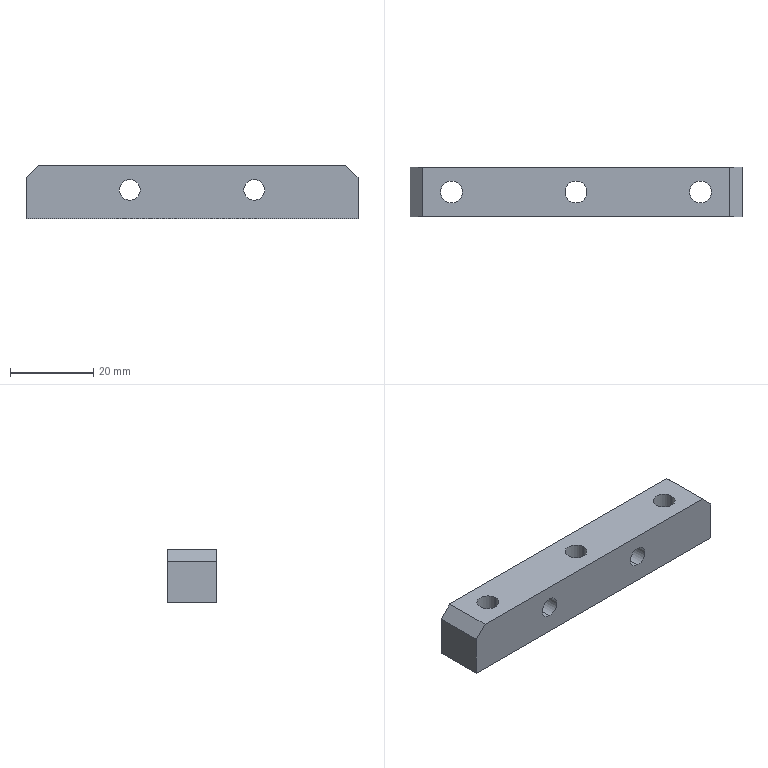Part | STEP file | PN_0013 | 1 solid | 18 faces | box 80 x 12 x 13 mm | volume 11040 mm3 | cylinder 10 | plane 8 | commonest cylinder face diameters 5.3 x6 5 x4
STEP:
#1=CARTESIAN_POINT('',(0.,0.,0.));
#2=DIRECTION('',(0.,0.,1.));
#3=DIRECTION('',(1.,0.,0.));
#4=AXIS2_PLACEMENT_3D('',#1,#2,#3);
#5=CARTESIAN_POINT('',(-15.,0.,3.));
#6=VERTEX_POINT('',#5);
#7=CARTESIAN_POINT('',(-15.,12.,3.));
#8=VERTEX_POINT('',#7);
#9=CARTESIAN_POINT('',(-15.,12.,3.));
#10=DIRECTION('',(0.,1.,0.));
#11=VECTOR('',#10,1.);
#12=LINE('',#9,#11);
#13=CARTESIAN_POINT('',(-15.,12.,0.5));
#14=DIRECTION('',(0.,1.,0.));
#15=DIRECTION('',(0.,0.,1.));
#16=AXIS2_PLACEMENT_3D('',#13,#14,#15);
#17=CYLINDRICAL_SURFACE('',#16,2.5);
#18=CARTESIAN_POINT('',(6.283,0.));
#19=DIRECTION('',(0.,1.));
#20=VECTOR('',#19,1.);
#21=LINE('',#18,#20);
#22=(GEOMETRIC_REPRESENTATION_CONTEXT(2)PARAMETRIC_REPRESENTATION_CONTEXT()REPRESENTATION_CONTEXT('',''));
#23=DEFINITIONAL_REPRESENTATION('',(#21),#22);
#24=PCURVE('',#17,#23);
#25=CARTESIAN_POINT('',(-15.,12.,0.5));
#26=DIRECTION('',(0.,1.,0.));
#27=DIRECTION('',(0.,0.,1.));
#28=AXIS2_PLACEMENT_3D('',#25,#26,#27);
#29=CYLINDRICAL_SURFACE('',#28,2.5);
#30=CARTESIAN_POINT('',(0.,0.));
#31=DIRECTION('',(0.,1.));
#32=VECTOR('',#31,1.);
#33=LINE('',#30,#32);
#34=(GEOMETRIC_REPRESENTATION_CONTEXT(2)PARAMETRIC_REPRESENTATION_CONTEXT()REPRESENTATION_CONTEXT('',''));
#35=DEFINITIONAL_REPRESENTATION('',(#33),#34);
#36=PCURVE('',#29,#35);
#37=SURFACE_CURVE('',#12,(#24,#36),.PCURVE_S1.);
#38=EDGE_CURVE('',#6,#8,#37,.T.);
#39=ORIENTED_EDGE('',*,*,#38,.T.);
#40=CARTESIAN_POINT('',(-15.,12.,-2.));
#41=VERTEX_POINT('',#40);
#42=CARTESIAN_POINT('',(-15.,12.,0.5));
#43=DIRECTION('',(0.,1.,0.));
#44=DIRECTION('',(0.,0.,1.));
#45=AXIS2_PLACEMENT_3D('',#42,#43,#44);
#46=CIRCLE('',#45,2.5);
#47=CARTESIAN_POINT('',(0.,0.));
#48=DIRECTION('',(1.,0.));
#49=VECTOR('',#48,1.);
#50=LINE('',#47,#49);
#51=(GEOMETRIC_REPRESENTATION_CONTEXT(2)PARAMETRIC_REPRESENTATION_CONTEXT()REPRESENTATION_CONTEXT('',''));
#52=DEFINITIONAL_REPRESENTATION('',(#50),#51);
#53=PCURVE('',#17,#52);
#54=CARTESIAN_POINT('',(0.,12.,0.));
#55=DIRECTION('',(0.,1.,0.));
#56=DIRECTION('',(0.,0.,1.));
#57=AXIS2_PLACEMENT_3D('',#54,#55,#56);
#58=PLANE('',#57);
#59=CARTESIAN_POINT('',(0.5,-15.));
#60=DIRECTION('',(1.,0.));
#61=AXIS2_PLACEMENT_2D('',#59,#60);
#62=CIRCLE('',#61,2.5);
#63=(GEOMETRIC_REPRESENTATION_CONTEXT(2)PARAMETRIC_REPRESENTATION_CONTEXT()REPRESENTATION_CONTEXT('',''));
#64=DEFINITIONAL_REPRESENTATION('',(#62),#63);
#65=PCURVE('',#58,#64);
#66=SURFACE_CURVE('',#46,(#53,#65),.PCURVE_S1.);
#67=EDGE_CURVE('',#41,#8,#66,.T.);
#68=ORIENTED_EDGE('',*,*,#67,.F.);
#69=CARTESIAN_POINT('',(-15.,0.,-2.));
#70=VERTEX_POINT('',#69);
#71=CARTESIAN_POINT('',(-15.,12.,-2.));
#72=DIRECTION('',(0.,1.,0.));
#73=VECTOR('',#72,1.);
#74=LINE('',#71,#73);
#75=CARTESIAN_POINT('',(3.142,0.));
#76=DIRECTION('',(0.,1.));
#77=VECTOR('',#76,1.);
#78=LINE('',#75,#77);
#79=(GEOMETRIC_REPRESENTATION_CONTEXT(2)PARAMETRIC_REPRESENTATION_CONTEXT()REPRESENTATION_CONTEXT('',''));
#80=DEFINITIONAL_REPRESENTATION('',(#78),#79);
#81=PCURVE('',#17,#80);
#82=CARTESIAN_POINT('',(3.142,0.));
#83=DIRECTION('',(0.,1.));
#84=VECTOR('',#83,1.);
#85=LINE('',#82,#84);
#86=(GEOMETRIC_REPRESENTATION_CONTEXT(2)PARAMETRIC_REPRESENTATION_CONTEXT()REPRESENTATION_CONTEXT('',''));
#87=DEFINITIONAL_REPRESENTATION('',(#85),#86);
#88=PCURVE('',#29,#87);
#89=SURFACE_CURVE('',#74,(#81,#88),.PCURVE_S1.);
#90=EDGE_CURVE('',#70,#41,#89,.T.);
#91=ORIENTED_EDGE('',*,*,#90,.F.);
#92=CARTESIAN_POINT('',(-15.,0.,0.5));
#93=DIRECTION('',(0.,1.,0.));
#94=DIRECTION('',(0.,0.,1.));
#95=AXIS2_PLACEMENT_3D('',#92,#93,#94);
#96=CIRCLE('',#95,2.5);
#97=CARTESIAN_POINT('',(0.,-12.));
#98=DIRECTION('',(1.,0.));
#99=VECTOR('',#98,1.);
#100=LINE('',#97,#99);
#101=(GEOMETRIC_REPRESENTATION_CONTEXT(2)PARAMETRIC_REPRESENTATION_CONTEXT()REPRESENTATION_CONTEXT('',''));
#102=DEFINITIONAL_REPRESENTATION('',(#100),#101);
#103=PCURVE('',#17,#102);
#104=CARTESIAN_POINT('',(0.,0.,0.));
#105=DIRECTION('',(0.,1.,0.));
#106=DIRECTION('',(0.,0.,1.));
#107=AXIS2_PLACEMENT_3D('',#104,#105,#106);
#108=PLANE('',#107);
#109=CARTESIAN_POINT('',(0.5,-15.));
#110=DIRECTION('',(1.,0.));
#111=AXIS2_PLACEMENT_2D('',#109,#110);
#112=CIRCLE('',#111,2.5);
#113=(GEOMETRIC_REPRESENTATION_CONTEXT(2)PARAMETRIC_REPRESENTATION_CONTEXT()REPRESENTATION_CONTEXT('',''));
#114=DEFINITIONAL_REPRESENTATION('',(#112),#113);
#115=PCURVE('',#108,#114);
#116=SURFACE_CURVE('',#96,(#103,#115),.PCURVE_S1.);
#117=EDGE_CURVE('',#70,#6,#116,.T.);
#118=ORIENTED_EDGE('',*,*,#117,.T.);
#119=EDGE_LOOP('',(#39,#68,#91,#118));
#120=FACE_BOUND('',#119,.F.);
#121=ADVANCED_FACE('',(#120),#17,.F.);
#122=CARTESIAN_POINT('',(15.,0.,3.));
#123=VERTEX_POINT('',#122);
#124=CARTESIAN_POINT('',(15.,12.,3.));
#125=VERTEX_POINT('',#124);
#126=CARTESIAN_POINT('',(15.,12.,3.));
#127=DIRECTION('',(0.,1.,0.));
#128=VECTOR('',#127,1.);
#129=LINE('',#126,#128);
#130=CARTESIAN_POINT('',(15.,12.,0.5));
#131=DIRECTION('',(0.,1.,0.));
#132=DIRECTION('',(0.,0.,1.));
#133=AXIS2_PLACEMENT_3D('',#130,#131,#132);
#134=CYLINDRICAL_SURFACE('',#133,2.5);
#135=CARTESIAN_POINT('',(6.283,0.));
#136=DIRECTION('',(0.,1.));
#137=VECTOR('',#136,1.);
#138=LINE('',#135,#137);
#139=(GEOMETRIC_REPRESENTATION_CONTEXT(2)PARAMETRIC_REPRESENTATION_CONTEXT()REPRESENTATION_CONTEXT('',''));
#140=DEFINITIONAL_REPRESENTATION('',(#138),#139);
#141=PCURVE('',#134,#140);
#142=CARTESIAN_POINT('',(15.,12.,0.5));
#143=DIRECTION('',(0.,1.,0.));
#144=DIRECTION('',(0.,0.,1.));
#145=AXIS2_PLACEMENT_3D('',#142,#143,#144);
#146=CYLINDRICAL_SURFACE('',#145,2.5);
#147=CARTESIAN_POINT('',(0.,0.));
#148=DIRECTION('',(0.,1.));
#149=VECTOR('',#148,1.);
#150=LINE('',#147,#149);
#151=(GEOMETRIC_REPRESENTATION_CONTEXT(2)PARAMETRIC_REPRESENTATION_CONTEXT()REPRESENTATION_CONTEXT('',''));
#152=DEFINITIONAL_REPRESENTATION('',(#150),#151);
#153=PCURVE('',#146,#152);
#154=SURFACE_CURVE('',#129,(#141,#153),.PCURVE_S1.);
#155=EDGE_CURVE('',#123,#125,#154,.T.);
#156=ORIENTED_EDGE('',*,*,#155,.T.);
#157=CARTESIAN_POINT('',(15.,12.,-2.));
#158=VERTEX_POINT('',#157);
#159=CARTESIAN_POINT('',(15.,12.,0.5));
#160=DIRECTION('',(0.,1.,0.));
#161=DIRECTION('',(0.,0.,1.));
#162=AXIS2_PLACEMENT_3D('',#159,#160,#161);
#163=CIRCLE('',#162,2.5);
#164=CARTESIAN_POINT('',(0.,0.));
#165=DIRECTION('',(1.,0.));
#166=VECTOR('',#165,1.);
#167=LINE('',#164,#166);
#168=(GEOMETRIC_REPRESENTATION_CONTEXT(2)PARAMETRIC_REPRESENTATION_CONTEXT()REPRESENTATION_CONTEXT('',''));
#169=DEFINITIONAL_REPRESENTATION('',(#167),#168);
#170=PCURVE('',#134,#169);
#171=CARTESIAN_POINT('',(0.5,15.));
#172=DIRECTION('',(1.,0.));
#173=AXIS2_PLACEMENT_2D('',#171,#172);
#174=CIRCLE('',#173,2.5);
#175=(GEOMETRIC_REPRESENTATION_CONTEXT(2)PARAMETRIC_REPRESENTATION_CONTEXT()REPRESENTATION_CONTEXT('',''));
#176=DEFINITIONAL_REPRESENTATION('',(#174),#175);
#177=PCURVE('',#58,#176);
#178=SURFACE_CURVE('',#163,(#170,#177),.PCURVE_S1.);
#179=EDGE_CURVE('',#158,#125,#178,.T.);
#180=ORIENTED_EDGE('',*,*,#179,.F.);
#181=CARTESIAN_POINT('',(15.,0.,-2.));
#182=VERTEX_POINT('',#181);
#183=CARTESIAN_POINT('',(15.,12.,-2.));
#184=DIRECTION('',(0.,1.,0.));
#185=VECTOR('',#184,1.);
#186=LINE('',#183,#185);
#187=CARTESIAN_POINT('',(3.142,0.));
#188=DIRECTION('',(0.,1.));
#189=VECTOR('',#188,1.);
#190=LINE('',#187,#189);
#191=(GEOMETRIC_REPRESENTATION_CONTEXT(2)PARAMETRIC_REPRESENTATION_CONTEXT()REPRESENTATION_CONTEXT('',''));
#192=DEFINITIONAL_REPRESENTATION('',(#190),#191);
#193=PCURVE('',#134,#192);
#194=CARTESIAN_POINT('',(3.142,0.));
#195=DIRECTION('',(0.,1.));
#196=VECTOR('',#195,1.);
#197=LINE('',#194,#196);
#198=(GEOMETRIC_REPRESENTATION_CONTEXT(2)PARAMETRIC_REPRESENTATION_CONTEXT()REPRESENTATION_CONTEXT('',''));
#199=DEFINITIONAL_REPRESENTATION('',(#197),#198);
#200=PCURVE('',#146,#199);
#201=SURFACE_CURVE('',#186,(#193,#200),.PCURVE_S1.);
#202=EDGE_CURVE('',#182,#158,#201,.T.);
#203=ORIENTED_EDGE('',*,*,#202,.F.);
#204=CARTESIAN_POINT('',(15.,0.,0.5));
#205=DIRECTION('',(0.,1.,0.));
#206=DIRECTION('',(0.,0.,1.));
#207=AXIS2_PLACEMENT_3D('',#204,#205,#206);
#208=CIRCLE('',#207,2.5);
#209=CARTESIAN_POINT('',(0.,-12.));
#210=DIRECTION('',(1.,0.));
#211=VECTOR('',#210,1.);
#212=LINE('',#209,#211);
#213=(GEOMETRIC_REPRESENTATION_CONTEXT(2)PARAMETRIC_REPRESENTATION_CONTEXT()REPRESENTATION_CONTEXT('',''));
#214=DEFINITIONAL_REPRESENTATION('',(#212),#213);
#215=PCURVE('',#134,#214);
#216=CARTESIAN_POINT('',(0.5,15.));
#217=DIRECTION('',(1.,0.));
#218=AXIS2_PLACEMENT_2D('',#216,#217);
#219=CIRCLE('',#218,2.5);
#220=(GEOMETRIC_REPRESENTATION_CONTEXT(2)PARAMETRIC_REPRESENTATION_CONTEXT()REPRESENTATION_CONTEXT('',''));
#221=DEFINITIONAL_REPRESENTATION('',(#219),#220);
#222=PCURVE('',#108,#221);
#223=SURFACE_CURVE('',#208,(#215,#222),.PCURVE_S1.);
#224=EDGE_CURVE('',#182,#123,#223,.T.);
#225=ORIENTED_EDGE('',*,*,#224,.T.);
#226=EDGE_LOOP('',(#156,#180,#203,#225));
#227=FACE_BOUND('',#226,.F.);
#228=ADVANCED_FACE('',(#227),#134,.F.);
#229=CARTESIAN_POINT('',(32.65,6.,-6.5));
#230=VERTEX_POINT('',#229);
#231=CARTESIAN_POINT('',(32.65,6.,6.5));
#232=VERTEX_POINT('',#231);
#233=CARTESIAN_POINT('',(32.65,6.,6.5));
#234=DIRECTION('',(0.,0.,1.));
#235=VECTOR('',#234,1.);
#236=LINE('',#233,#235);
#237=CARTESIAN_POINT('',(30.,6.,6.5));
#238=DIRECTION('',(0.,0.,1.));
#239=DIRECTION('',(1.,0.,0.));
#240=AXIS2_PLACEMENT_3D('',#237,#238,#239);
#241=CYLINDRICAL_SURFACE('',#240,2.65);
#242=CARTESIAN_POINT('',(6.283,0.));
#243=DIRECTION('',(0.,1.));
#244=VECTOR('',#243,1.);
#245=LINE('',#242,#244);
#246=(GEOMETRIC_REPRESENTATION_CONTEXT(2)PARAMETRIC_REPRESENTATION_CONTEXT()REPRESENTATION_CONTEXT('',''));
#247=DEFINITIONAL_REPRESENTATION('',(#245),#246);
#248=PCURVE('',#241,#247);
#249=CARTESIAN_POINT('',(30.,6.,6.5));
#250=DIRECTION('',(0.,0.,1.));
#251=DIRECTION('',(1.,0.,0.));
#252=AXIS2_PLACEMENT_3D('',#249,#250,#251);
#253=CYLINDRICAL_SURFACE('',#252,2.65);
#254=CARTESIAN_POINT('',(0.,0.));
#255=DIRECTION('',(0.,1.));
#256=VECTOR('',#255,1.);
#257=LINE('',#254,#256);
#258=(GEOMETRIC_REPRESENTATION_CONTEXT(2)PARAMETRIC_REPRESENTATION_CONTEXT()REPRESENTATION_CONTEXT('',''));
#259=DEFINITIONAL_REPRESENTATION('',(#257),#258);
#260=PCURVE('',#253,#259);
#261=SURFACE_CURVE('',#236,(#248,#260),.PCURVE_S1.);
#262=EDGE_CURVE('',#230,#232,#261,.T.);
#263=ORIENTED_EDGE('',*,*,#262,.T.);
#264=CARTESIAN_POINT('',(27.35,6.,6.5));
#265=VERTEX_POINT('',#264);
#266=CARTESIAN_POINT('',(30.,6.,6.5));
#267=DIRECTION('',(0.,0.,1.));
#268=DIRECTION('',(1.,0.,0.));
#269=AXIS2_PLACEMENT_3D('',#266,#267,#268);
#270=CIRCLE('',#269,2.65);
#271=CARTESIAN_POINT('',(0.,0.));
#272=DIRECTION('',(1.,0.));
#273=VECTOR('',#272,1.);
#274=LINE('',#271,#273);
#275=(GEOMETRIC_REPRESENTATION_CONTEXT(2)PARAMETRIC_REPRESENTATION_CONTEXT()REPRESENTATION_CONTEXT('',''));
#276=DEFINITIONAL_REPRESENTATION('',(#274),#275);
#277=PCURVE('',#241,#276);
#278=CARTESIAN_POINT('',(-40.,12.,6.5));
#279=DIRECTION('',(0.,0.,-1.));
#280=DIRECTION('',(-1.,0.,0.));
#281=AXIS2_PLACEMENT_3D('',#278,#279,#280);
#282=PLANE('',#281);
#283=CARTESIAN_POINT('',(-72.65,-6.));
#284=CARTESIAN_POINT('',(-72.65,-1.41));
#285=CARTESIAN_POINT('',(-68.675,-3.705));
#286=CARTESIAN_POINT('',(-64.7,-6.));
#287=CARTESIAN_POINT('',(-68.675,-8.295));
#288=CARTESIAN_POINT('',(-72.65,-10.59));
#289=CARTESIAN_POINT('',(-72.65,-6.));
#290=(BOUNDED_CURVE()B_SPLINE_CURVE(2,(#283,#284,#285,#286,#287,#288,#289),.UNSPECIFIED.,.T.,.F.)B_SPLINE_CURVE_WITH_KNOTS((1,2,2,2,2,1),(-2.094,0.,2.094,4.189,6.283,8.378),.UNSPECIFIED.)CURVE()GEOMETRIC_REPRESENTATION_ITEM()RATIONAL_B_SPLINE_CURVE((1.,0.5,1.,0.5,1.,0.5,1.))REPRESENTATION_ITEM(''));
#291=(GEOMETRIC_REPRESENTATION_CONTEXT(2)PARAMETRIC_REPRESENTATION_CONTEXT()REPRESENTATION_CONTEXT('',''));
#292=DEFINITIONAL_REPRESENTATION('',(#290),#291);
#293=PCURVE('',#282,#292);
#294=SURFACE_CURVE('',#270,(#277,#293),.PCURVE_S1.);
#295=EDGE_CURVE('',#265,#232,#294,.T.);
#296=ORIENTED_EDGE('',*,*,#295,.F.);
#297=CARTESIAN_POINT('',(27.35,6.,-6.5));
#298=VERTEX_POINT('',#297);
#299=CARTESIAN_POINT('',(27.35,6.,6.5));
#300=DIRECTION('',(0.,0.,1.));
#301=VECTOR('',#300,1.);
#302=LINE('',#299,#301);
#303=CARTESIAN_POINT('',(3.142,0.));
#304=DIRECTION('',(0.,1.));
#305=VECTOR('',#304,1.);
#306=LINE('',#303,#305);
#307=(GEOMETRIC_REPRESENTATION_CONTEXT(2)PARAMETRIC_REPRESENTATION_CONTEXT()REPRESENTATION_CONTEXT('',''));
#308=DEFINITIONAL_REPRESENTATION('',(#306),#307);
#309=PCURVE('',#241,#308);
#310=CARTESIAN_POINT('',(3.142,0.));
#311=DIRECTION('',(0.,1.));
#312=VECTOR('',#311,1.);
#313=LINE('',#310,#312);
#314=(GEOMETRIC_REPRESENTATION_CONTEXT(2)PARAMETRIC_REPRESENTATION_CONTEXT()REPRESENTATION_CONTEXT('',''));
#315=DEFINITIONAL_REPRESENTATION('',(#313),#314);
#316=PCURVE('',#253,#315);
#317=SURFACE_CURVE('',#302,(#309,#316),.PCURVE_S1.);
#318=EDGE_CURVE('',#298,#265,#317,.T.);
#319=ORIENTED_EDGE('',*,*,#318,.F.);
#320=CARTESIAN_POINT('',(30.,6.,-6.5));
#321=DIRECTION('',(0.,0.,1.));
#322=DIRECTION('',(1.,0.,0.));
#323=AXIS2_PLACEMENT_3D('',#320,#321,#322);
#324=CIRCLE('',#323,2.65);
#325=CARTESIAN_POINT('',(0.,-13.));
#326=DIRECTION('',(1.,0.));
#327=VECTOR('',#326,1.);
#328=LINE('',#325,#327);
#329=(GEOMETRIC_REPRESENTATION_CONTEXT(2)PARAMETRIC_REPRESENTATION_CONTEXT()REPRESENTATION_CONTEXT('',''));
#330=DEFINITIONAL_REPRESENTATION('',(#328),#329);
#331=PCURVE('',#241,#330);
#332=CARTESIAN_POINT('',(-40.,12.,-6.5));
#333=DIRECTION('',(0.,0.,1.));
#334=DIRECTION('',(1.,0.,0.));
#335=AXIS2_PLACEMENT_3D('',#332,#333,#334);
#336=PLANE('',#335);
#337=CARTESIAN_POINT('',(70.,-6.));
#338=DIRECTION('',(1.,0.));
#339=AXIS2_PLACEMENT_2D('',#337,#338);
#340=CIRCLE('',#339,2.65);
#341=(GEOMETRIC_REPRESENTATION_CONTEXT(2)PARAMETRIC_REPRESENTATION_CONTEXT()REPRESENTATION_CONTEXT('',''));
#342=DEFINITIONAL_REPRESENTATION('',(#340),#341);
#343=PCURVE('',#336,#342);
#344=SURFACE_CURVE('',#324,(#331,#343),.PCURVE_S1.);
#345=EDGE_CURVE('',#298,#230,#344,.T.);
#346=ORIENTED_EDGE('',*,*,#345,.T.);
#347=EDGE_LOOP('',(#263,#296,#319,#346));
#348=FACE_BOUND('',#347,.F.);
#349=ADVANCED_FACE('',(#348),#241,.F.);
#350=CARTESIAN_POINT('',(2.65,6.,-6.5));
#351=VERTEX_POINT('',#350);
#352=CARTESIAN_POINT('',(2.65,6.,6.5));
#353=VERTEX_POINT('',#352);
#354=CARTESIAN_POINT('',(2.65,6.,6.5));
#355=DIRECTION('',(0.,0.,1.));
#356=VECTOR('',#355,1.);
#357=LINE('',#354,#356);
#358=CARTESIAN_POINT('',(0.,6.,6.5));
#359=DIRECTION('',(0.,0.,1.));
#360=DIRECTION('',(1.,0.,0.));
#361=AXIS2_PLACEMENT_3D('',#358,#359,#360);
#362=CYLINDRICAL_SURFACE('',#361,2.65);
#363=CARTESIAN_POINT('',(6.283,0.));
#364=DIRECTION('',(0.,1.));
#365=VECTOR('',#364,1.);
#366=LINE('',#363,#365);
#367=(GEOMETRIC_REPRESENTATION_CONTEXT(2)PARAMETRIC_REPRESENTATION_CONTEXT()REPRESENTATION_CONTEXT('',''));
#368=DEFINITIONAL_REPRESENTATION('',(#366),#367);
#369=PCURVE('',#362,#368);
#370=CARTESIAN_POINT('',(0.,6.,6.5));
#371=DIRECTION('',(0.,0.,1.));
#372=DIRECTION('',(1.,0.,0.));
#373=AXIS2_PLACEMENT_3D('',#370,#371,#372);
#374=CYLINDRICAL_SURFACE('',#373,2.65);
#375=CARTESIAN_POINT('',(0.,0.));
#376=DIRECTION('',(0.,1.));
#377=VECTOR('',#376,1.);
#378=LINE('',#375,#377);
#379=(GEOMETRIC_REPRESENTATION_CONTEXT(2)PARAMETRIC_REPRESENTATION_CONTEXT()REPRESENTATION_CONTEXT('',''));
#380=DEFINITIONAL_REPRESENTATION('',(#378),#379);
#381=PCURVE('',#374,#380);
#382=SURFACE_CURVE('',#357,(#369,#381),.PCURVE_S1.);
#383=EDGE_CURVE('',#351,#353,#382,.T.);
#384=ORIENTED_EDGE('',*,*,#383,.T.);
#385=CARTESIAN_POINT('',(-2.65,6.,6.5));
#386=VERTEX_POINT('',#385);
#387=CARTESIAN_POINT('',(0.,6.,6.5));
#388=DIRECTION('',(0.,0.,1.));
#389=DIRECTION('',(1.,0.,0.));
#390=AXIS2_PLACEMENT_3D('',#387,#388,#389);
#391=CIRCLE('',#390,2.65);
#392=CARTESIAN_POINT('',(0.,0.));
#393=DIRECTION('',(1.,0.));
#394=VECTOR('',#393,1.);
#395=LINE('',#392,#394);
#396=(GEOMETRIC_REPRESENTATION_CONTEXT(2)PARAMETRIC_REPRESENTATION_CONTEXT()REPRESENTATION_CONTEXT('',''));
#397=DEFINITIONAL_REPRESENTATION('',(#395),#396);
#398=PCURVE('',#362,#397);
#399=CARTESIAN_POINT('',(-42.65,-6.));
#400=CARTESIAN_POINT('',(-42.65,-1.41));
#401=CARTESIAN_POINT('',(-38.675,-3.705));
#402=CARTESIAN_POINT('',(-34.7,-6.));
#403=CARTESIAN_POINT('',(-38.675,-8.295));
#404=CARTESIAN_POINT('',(-42.65,-10.59));
#405=CARTESIAN_POINT('',(-42.65,-6.));
#406=(BOUNDED_CURVE()B_SPLINE_CURVE(2,(#399,#400,#401,#402,#403,#404,#405),.UNSPECIFIED.,.T.,.F.)B_SPLINE_CURVE_WITH_KNOTS((1,2,2,2,2,1),(-2.094,0.,2.094,4.189,6.283,8.378),.UNSPECIFIED.)CURVE()GEOMETRIC_REPRESENTATION_ITEM()RATIONAL_B_SPLINE_CURVE((1.,0.5,1.,0.5,1.,0.5,1.))REPRESENTATION_ITEM(''));
#407=(GEOMETRIC_REPRESENTATION_CONTEXT(2)PARAMETRIC_REPRESENTATION_CONTEXT()REPRESENTATION_CONTEXT('',''));
#408=DEFINITIONAL_REPRESENTATION('',(#406),#407);
#409=PCURVE('',#282,#408);
#410=SURFACE_CURVE('',#391,(#398,#409),.PCURVE_S1.);
#411=EDGE_CURVE('',#386,#353,#410,.T.);
#412=ORIENTED_EDGE('',*,*,#411,.F.);
#413=CARTESIAN_POINT('',(-2.65,6.,-6.5));
#414=VERTEX_POINT('',#413);
#415=CARTESIAN_POINT('',(-2.65,6.,6.5));
#416=DIRECTION('',(0.,0.,1.));
#417=VECTOR('',#416,1.);
#418=LINE('',#415,#417);
#419=CARTESIAN_POINT('',(3.142,0.));
#420=DIRECTION('',(0.,1.));
#421=VECTOR('',#420,1.);
#422=LINE('',#419,#421);
#423=(GEOMETRIC_REPRESENTATION_CONTEXT(2)PARAMETRIC_REPRESENTATION_CONTEXT()REPRESENTATION_CONTEXT('',''));
#424=DEFINITIONAL_REPRESENTATION('',(#422),#423);
#425=PCURVE('',#362,#424);
#426=CARTESIAN_POINT('',(3.142,0.));
#427=DIRECTION('',(0.,1.));
#428=VECTOR('',#427,1.);
#429=LINE('',#426,#428);
#430=(GEOMETRIC_REPRESENTATION_CONTEXT(2)PARAMETRIC_REPRESENTATION_CONTEXT()REPRESENTATION_CONTEXT('',''));
#431=DEFINITIONAL_REPRESENTATION('',(#429),#430);
#432=PCURVE('',#374,#431);
#433=SURFACE_CURVE('',#418,(#425,#432),.PCURVE_S1.);
#434=EDGE_CURVE('',#414,#386,#433,.T.);
#435=ORIENTED_EDGE('',*,*,#434,.F.);
#436=CARTESIAN_POINT('',(0.,6.,-6.5));
#437=DIRECTION('',(0.,0.,1.));
#438=DIRECTION('',(1.,0.,0.));
#439=AXIS2_PLACEMENT_3D('',#436,#437,#438);
#440=CIRCLE('',#439,2.65);
#441=CARTESIAN_POINT('',(0.,-13.));
#442=DIRECTION('',(1.,0.));
#443=VECTOR('',#442,1.);
#444=LINE('',#441,#443);
#445=(GEOMETRIC_REPRESENTATION_CONTEXT(2)PARAMETRIC_REPRESENTATION_CONTEXT()REPRESENTATION_CONTEXT('',''));
#446=DEFINITIONAL_REPRESENTATION('',(#444),#445);
#447=PCURVE('',#362,#446);
#448=CARTESIAN_POINT('',(40.,-6.));
#449=DIRECTION('',(1.,0.));
#450=AXIS2_PLACEMENT_2D('',#448,#449);
#451=CIRCLE('',#450,2.65);
#452=(GEOMETRIC_REPRESENTATION_CONTEXT(2)PARAMETRIC_REPRESENTATION_CONTEXT()REPRESENTATION_CONTEXT('',''));
#453=DEFINITIONAL_REPRESENTATION('',(#451),#452);
#454=PCURVE('',#336,#453);
#455=SURFACE_CURVE('',#440,(#447,#454),.PCURVE_S1.);
#456=EDGE_CURVE('',#414,#351,#455,.T.);
#457=ORIENTED_EDGE('',*,*,#456,.T.);
#458=EDGE_LOOP('',(#384,#412,#435,#457));
#459=FACE_BOUND('',#458,.F.);
#460=ADVANCED_FACE('',(#459),#362,.F.);
#461=CARTESIAN_POINT('',(-27.35,6.,-6.5));
#462=VERTEX_POINT('',#461);
#463=CARTESIAN_POINT('',(-27.35,6.,6.5));
#464=VERTEX_POINT('',#463);
#465=CARTESIAN_POINT('',(-27.35,6.,6.5));
#466=DIRECTION('',(0.,0.,1.));
#467=VECTOR('',#466,1.);
#468=LINE('',#465,#467);
#469=CARTESIAN_POINT('',(-30.,6.,6.5));
#470=DIRECTION('',(0.,0.,1.));
#471=DIRECTION('',(1.,0.,0.));
#472=AXIS2_PLACEMENT_3D('',#469,#470,#471);
#473=CYLINDRICAL_SURFACE('',#472,2.65);
#474=CARTESIAN_POINT('',(6.283,0.));
#475=DIRECTION('',(0.,1.));
#476=VECTOR('',#475,1.);
#477=LINE('',#474,#476);
#478=(GEOMETRIC_REPRESENTATION_CONTEXT(2)PARAMETRIC_REPRESENTATION_CONTEXT()REPRESENTATION_CONTEXT('',''));
#479=DEFINITIONAL_REPRESENTATION('',(#477),#478);
#480=PCURVE('',#473,#479);
#481=CARTESIAN_POINT('',(-30.,6.,6.5));
#482=DIRECTION('',(0.,0.,1.));
#483=DIRECTION('',(1.,0.,0.));
#484=AXIS2_PLACEMENT_3D('',#481,#482,#483);
#485=CYLINDRICAL_SURFACE('',#484,2.65);
#486=CARTESIAN_POINT('',(0.,0.));
#487=DIRECTION('',(0.,1.));
#488=VECTOR('',#487,1.);
#489=LINE('',#486,#488);
#490=(GEOMETRIC_REPRESENTATION_CONTEXT(2)PARAMETRIC_REPRESENTATION_CONTEXT()REPRESENTATION_CONTEXT('',''));
#491=DEFINITIONAL_REPRESENTATION('',(#489),#490);
#492=PCURVE('',#485,#491);
#493=SURFACE_CURVE('',#468,(#480,#492),.PCURVE_S1.);
#494=EDGE_CURVE('',#462,#464,#493,.T.);
#495=ORIENTED_EDGE('',*,*,#494,.T.);
#496=CARTESIAN_POINT('',(-32.65,6.,6.5));
#497=VERTEX_POINT('',#496);
#498=CARTESIAN_POINT('',(-30.,6.,6.5));
#499=DIRECTION('',(0.,0.,1.));
#500=DIRECTION('',(1.,0.,0.));
#501=AXIS2_PLACEMENT_3D('',#498,#499,#500);
#502=CIRCLE('',#501,2.65);
#503=CARTESIAN_POINT('',(0.,0.));
#504=DIRECTION('',(1.,0.));
#505=VECTOR('',#504,1.);
#506=LINE('',#503,#505);
#507=(GEOMETRIC_REPRESENTATION_CONTEXT(2)PARAMETRIC_REPRESENTATION_CONTEXT()REPRESENTATION_CONTEXT('',''));
#508=DEFINITIONAL_REPRESENTATION('',(#506),#507);
#509=PCURVE('',#473,#508);
#510=CARTESIAN_POINT('',(-12.65,-6.));
#511=CARTESIAN_POINT('',(-12.65,-1.41));
#512=CARTESIAN_POINT('',(-8.675,-3.705));
#513=CARTESIAN_POINT('',(-4.7,-6.));
#514=CARTESIAN_POINT('',(-8.675,-8.295));
#515=CARTESIAN_POINT('',(-12.65,-10.59));
#516=CARTESIAN_POINT('',(-12.65,-6.));
#517=(BOUNDED_CURVE()B_SPLINE_CURVE(2,(#510,#511,#512,#513,#514,#515,#516),.UNSPECIFIED.,.T.,.F.)B_SPLINE_CURVE_WITH_KNOTS((1,2,2,2,2,1),(-2.094,0.,2.094,4.189,6.283,8.378),.UNSPECIFIED.)CURVE()GEOMETRIC_REPRESENTATION_ITEM()RATIONAL_B_SPLINE_CURVE((1.,0.5,1.,0.5,1.,0.5,1.))REPRESENTATION_ITEM(''));
#518=(GEOMETRIC_REPRESENTATION_CONTEXT(2)PARAMETRIC_REPRESENTATION_CONTEXT()REPRESENTATION_CONTEXT('',''));
#519=DEFINITIONAL_REPRESENTATION('',(#517),#518);
#520=PCURVE('',#282,#519);
#521=SURFACE_CURVE('',#502,(#509,#520),.PCURVE_S1.);
#522=EDGE_CURVE('',#497,#464,#521,.T.);
#523=ORIENTED_EDGE('',*,*,#522,.F.);
#524=CARTESIAN_POINT('',(-32.65,6.,-6.5));
#525=VERTEX_POINT('',#524);
#526=CARTESIAN_POINT('',(-32.65,6.,6.5));
#527=DIRECTION('',(0.,0.,1.));
#528=VECTOR('',#527,1.);
#529=LINE('',#526,#528);
#530=CARTESIAN_POINT('',(3.142,0.));
#531=DIRECTION('',(0.,1.));
#532=VECTOR('',#531,1.);
#533=LINE('',#530,#532);
#534=(GEOMETRIC_REPRESENTATION_CONTEXT(2)PARAMETRIC_REPRESENTATION_CONTEXT()REPRESENTATION_CONTEXT('',''));
#535=DEFINITIONAL_REPRESENTATION('',(#533),#534);
#536=PCURVE('',#473,#535);
#537=CARTESIAN_POINT('',(3.142,0.));
#538=DIRECTION('',(0.,1.));
#539=VECTOR('',#538,1.);
#540=LINE('',#537,#539);
#541=(GEOMETRIC_REPRESENTATION_CONTEXT(2)PARAMETRIC_REPRESENTATION_CONTEXT()REPRESENTATION_CONTEXT('',''));
#542=DEFINITIONAL_REPRESENTATION('',(#540),#541);
#543=PCURVE('',#485,#542);
#544=SURFACE_CURVE('',#529,(#536,#543),.PCURVE_S1.);
#545=EDGE_CURVE('',#525,#497,#544,.T.);
#546=ORIENTED_EDGE('',*,*,#545,.F.);
#547=CARTESIAN_POINT('',(-30.,6.,-6.5));
#548=DIRECTION('',(0.,0.,1.));
#549=DIRECTION('',(1.,0.,0.));
#550=AXIS2_PLACEMENT_3D('',#547,#548,#549);
#551=CIRCLE('',#550,2.65);
#552=CARTESIAN_POINT('',(0.,-13.));
#553=DIRECTION('',(1.,0.));
#554=VECTOR('',#553,1.);
#555=LINE('',#552,#554);
#556=(GEOMETRIC_REPRESENTATION_CONTEXT(2)PARAMETRIC_REPRESENTATION_CONTEXT()REPRESENTATION_CONTEXT('',''));
#557=DEFINITIONAL_REPRESENTATION('',(#555),#556);
#558=PCURVE('',#473,#557);
#559=CARTESIAN_POINT('',(10.,-6.));
#560=DIRECTION('',(1.,0.));
#561=AXIS2_PLACEMENT_2D('',#559,#560);
#562=CIRCLE('',#561,2.65);
#563=(GEOMETRIC_REPRESENTATION_CONTEXT(2)PARAMETRIC_REPRESENTATION_CONTEXT()REPRESENTATION_CONTEXT('',''));
#564=DEFINITIONAL_REPRESENTATION('',(#562),#563);
#565=PCURVE('',#336,#564);
#566=SURFACE_CURVE('',#551,(#558,#565),.PCURVE_S1.);
#567=EDGE_CURVE('',#525,#462,#566,.T.);
#568=ORIENTED_EDGE('',*,*,#567,.T.);
#569=EDGE_LOOP('',(#495,#523,#546,#568));
#570=FACE_BOUND('',#569,.F.);
#571=ADVANCED_FACE('',(#570),#473,.F.);
#572=CARTESIAN_POINT('',(40.,12.,3.5));
#573=VERTEX_POINT('',#572);
#574=CARTESIAN_POINT('',(40.,12.,-6.5));
#575=VERTEX_POINT('',#574);
#576=CARTESIAN_POINT('',(40.,12.,-6.5));
#577=DIRECTION('',(0.,0.,-1.));
#578=VECTOR('',#577,1.);
#579=LINE('',#576,#578);
#580=CARTESIAN_POINT('',(40.,12.,-6.5));
#581=DIRECTION('',(-1.,0.,0.));
#582=DIRECTION('',(0.,0.,1.));
#583=AXIS2_PLACEMENT_3D('',#580,#581,#582);
#584=PLANE('',#583);
#585=CARTESIAN_POINT('',(0.,0.));
#586=DIRECTION('',(-1.,0.));
#587=VECTOR('',#586,1.);
#588=LINE('',#585,#587);
#589=(GEOMETRIC_REPRESENTATION_CONTEXT(2)PARAMETRIC_REPRESENTATION_CONTEXT()REPRESENTATION_CONTEXT('',''));
#590=DEFINITIONAL_REPRESENTATION('',(#588),#589);
#591=PCURVE('',#584,#590);
#592=CARTESIAN_POINT('',(-6.5,40.));
#593=DIRECTION('',(-1.,0.));
#594=VECTOR('',#593,1.);
#595=LINE('',#592,#594);
#596=(GEOMETRIC_REPRESENTATION_CONTEXT(2)PARAMETRIC_REPRESENTATION_CONTEXT()REPRESENTATION_CONTEXT('',''));
#597=DEFINITIONAL_REPRESENTATION('',(#595),#596);
#598=PCURVE('',#58,#597);
#599=SURFACE_CURVE('',#579,(#591,#598),.PCURVE_S1.);
#600=EDGE_CURVE('',#573,#575,#599,.T.);
#601=ORIENTED_EDGE('',*,*,#600,.F.);
#602=CARTESIAN_POINT('',(40.,0.,3.5));
#603=VERTEX_POINT('',#602);
#604=CARTESIAN_POINT('',(40.,12.,3.5));
#605=DIRECTION('',(0.,-1.,0.));
#606=VECTOR('',#605,1.);
#607=LINE('',#604,#606);
#608=CARTESIAN_POINT('',(10.,0.));
#609=DIRECTION('',(0.,-1.));
#610=VECTOR('',#609,1.);
#611=LINE('',#608,#610);
#612=(GEOMETRIC_REPRESENTATION_CONTEXT(2)PARAMETRIC_REPRESENTATION_CONTEXT()REPRESENTATION_CONTEXT('',''));
#613=DEFINITIONAL_REPRESENTATION('',(#611),#612);
#614=PCURVE('',#584,#613);
#615=CARTESIAN_POINT('',(40.,12.,3.5));
#616=DIRECTION('',(-0.7071,0.,-0.7071));
#617=DIRECTION('',(0.,-1.,0.));
#618=AXIS2_PLACEMENT_3D('',#615,#616,#617);
#619=PLANE('',#618);
#620=CARTESIAN_POINT('',(0.,0.));
#621=DIRECTION('',(1.,0.));
#622=VECTOR('',#621,1.);
#623=LINE('',#620,#622);
#624=(GEOMETRIC_REPRESENTATION_CONTEXT(2)PARAMETRIC_REPRESENTATION_CONTEXT()REPRESENTATION_CONTEXT('',''));
#625=DEFINITIONAL_REPRESENTATION('',(#623),#624);
#626=PCURVE('',#619,#625);
#627=SURFACE_CURVE('',#607,(#614,#626),.PCURVE_S1.);
#628=EDGE_CURVE('',#573,#603,#627,.T.);
#629=ORIENTED_EDGE('',*,*,#628,.T.);
#630=CARTESIAN_POINT('',(40.,0.,-6.5));
#631=VERTEX_POINT('',#630);
#632=CARTESIAN_POINT('',(40.,0.,-6.5));
#633=DIRECTION('',(0.,0.,-1.));
#634=VECTOR('',#633,1.);
#635=LINE('',#632,#634);
#636=CARTESIAN_POINT('',(0.,-12.));
#637=DIRECTION('',(-1.,0.));
#638=VECTOR('',#637,1.);
#639=LINE('',#636,#638);
#640=(GEOMETRIC_REPRESENTATION_CONTEXT(2)PARAMETRIC_REPRESENTATION_CONTEXT()REPRESENTATION_CONTEXT('',''));
#641=DEFINITIONAL_REPRESENTATION('',(#639),#640);
#642=PCURVE('',#584,#641);
#643=CARTESIAN_POINT('',(-6.5,40.));
#644=DIRECTION('',(-1.,0.));
#645=VECTOR('',#644,1.);
#646=LINE('',#643,#645);
#647=(GEOMETRIC_REPRESENTATION_CONTEXT(2)PARAMETRIC_REPRESENTATION_CONTEXT()REPRESENTATION_CONTEXT('',''));
#648=DEFINITIONAL_REPRESENTATION('',(#646),#647);
#649=PCURVE('',#108,#648);
#650=SURFACE_CURVE('',#635,(#642,#649),.PCURVE_S1.);
#651=EDGE_CURVE('',#603,#631,#650,.T.);
#652=ORIENTED_EDGE('',*,*,#651,.T.);
#653=CARTESIAN_POINT('',(40.,12.,-6.5));
#654=DIRECTION('',(0.,-1.,0.));
#655=VECTOR('',#654,1.);
#656=LINE('',#653,#655);
#657=CARTESIAN_POINT('',(0.,0.));
#658=DIRECTION('',(0.,-1.));
#659=VECTOR('',#658,1.);
#660=LINE('',#657,#659);
#661=(GEOMETRIC_REPRESENTATION_CONTEXT(2)PARAMETRIC_REPRESENTATION_CONTEXT()REPRESENTATION_CONTEXT('',''));
#662=DEFINITIONAL_REPRESENTATION('',(#660),#661);
#663=PCURVE('',#584,#662);
#664=CARTESIAN_POINT('',(80.,0.));
#665=DIRECTION('',(0.,-1.));
#666=VECTOR('',#665,1.);
#667=LINE('',#664,#666);
#668=(GEOMETRIC_REPRESENTATION_CONTEXT(2)PARAMETRIC_REPRESENTATION_CONTEXT()REPRESENTATION_CONTEXT('',''));
#669=DEFINITIONAL_REPRESENTATION('',(#667),#668);
#670=PCURVE('',#336,#669);
#671=SURFACE_CURVE('',#656,(#663,#670),.PCURVE_S1.);
#672=EDGE_CURVE('',#575,#631,#671,.T.);
#673=ORIENTED_EDGE('',*,*,#672,.F.);
#674=EDGE_LOOP('',(#601,#629,#652,#673));
#675=FACE_BOUND('',#674,.T.);
#676=ADVANCED_FACE('',(#675),#584,.F.);
#677=CARTESIAN_POINT('',(30.,6.,-6.5));
#678=DIRECTION('',(0.,0.,1.));
#679=DIRECTION('',(1.,0.,0.));
#680=AXIS2_PLACEMENT_3D('',#677,#678,#679);
#681=CIRCLE('',#680,2.65);
#682=CARTESIAN_POINT('',(70.,-6.));
#683=DIRECTION('',(1.,0.));
#684=AXIS2_PLACEMENT_2D('',#682,#683);
#685=CIRCLE('',#684,2.65);
#686=(GEOMETRIC_REPRESENTATION_CONTEXT(2)PARAMETRIC_REPRESENTATION_CONTEXT()REPRESENTATION_CONTEXT('',''));
#687=DEFINITIONAL_REPRESENTATION('',(#685),#686);
#688=PCURVE('',#336,#687);
#689=CARTESIAN_POINT('',(0.,-13.));
#690=DIRECTION('',(1.,0.));
#691=VECTOR('',#690,1.);
#692=LINE('',#689,#691);
#693=(GEOMETRIC_REPRESENTATION_CONTEXT(2)PARAMETRIC_REPRESENTATION_CONTEXT()REPRESENTATION_CONTEXT('',''));
#694=DEFINITIONAL_REPRESENTATION('',(#692),#693);
#695=PCURVE('',#253,#694);
#696=SURFACE_CURVE('',#681,(#688,#695),.PCURVE_S1.);
#697=EDGE_CURVE('',#230,#298,#696,.T.);
#698=ORIENTED_EDGE('',*,*,#697,.T.);
#699=ORIENTED_EDGE('',*,*,#345,.T.);
#700=EDGE_LOOP('',(#698,#699));
#701=FACE_BOUND('',#700,.T.);
#702=CARTESIAN_POINT('',(0.,6.,-6.5));
#703=DIRECTION('',(0.,0.,1.));
#704=DIRECTION('',(1.,0.,0.));
#705=AXIS2_PLACEMENT_3D('',#702,#703,#704);
#706=CIRCLE('',#705,2.65);
#707=CARTESIAN_POINT('',(40.,-6.));
#708=DIRECTION('',(1.,0.));
#709=AXIS2_PLACEMENT_2D('',#707,#708);
#710=CIRCLE('',#709,2.65);
#711=(GEOMETRIC_REPRESENTATION_CONTEXT(2)PARAMETRIC_REPRESENTATION_CONTEXT()REPRESENTATION_CONTEXT('',''));
#712=DEFINITIONAL_REPRESENTATION('',(#710),#711);
#713=PCURVE('',#336,#712);
#714=CARTESIAN_POINT('',(0.,-13.));
#715=DIRECTION('',(1.,0.));
#716=VECTOR('',#715,1.);
#717=LINE('',#714,#716);
#718=(GEOMETRIC_REPRESENTATION_CONTEXT(2)PARAMETRIC_REPRESENTATION_CONTEXT()REPRESENTATION_CONTEXT('',''));
#719=DEFINITIONAL_REPRESENTATION('',(#717),#718);
#720=PCURVE('',#374,#719);
#721=SURFACE_CURVE('',#706,(#713,#720),.PCURVE_S1.);
#722=EDGE_CURVE('',#351,#414,#721,.T.);
#723=ORIENTED_EDGE('',*,*,#722,.T.);
#724=ORIENTED_EDGE('',*,*,#456,.T.);
#725=EDGE_LOOP('',(#723,#724));
#726=FACE_BOUND('',#725,.T.);
#727=CARTESIAN_POINT('',(-30.,6.,-6.5));
#728=DIRECTION('',(0.,0.,1.));
#729=DIRECTION('',(1.,0.,0.));
#730=AXIS2_PLACEMENT_3D('',#727,#728,#729);
#731=CIRCLE('',#730,2.65);
#732=CARTESIAN_POINT('',(10.,-6.));
#733=DIRECTION('',(1.,0.));
#734=AXIS2_PLACEMENT_2D('',#732,#733);
#735=CIRCLE('',#734,2.65);
#736=(GEOMETRIC_REPRESENTATION_CONTEXT(2)PARAMETRIC_REPRESENTATION_CONTEXT()REPRESENTATION_CONTEXT('',''));
#737=DEFINITIONAL_REPRESENTATION('',(#735),#736);
#738=PCURVE('',#336,#737);
#739=CARTESIAN_POINT('',(0.,-13.));
#740=DIRECTION('',(1.,0.));
#741=VECTOR('',#740,1.);
#742=LINE('',#739,#741);
#743=(GEOMETRIC_REPRESENTATION_CONTEXT(2)PARAMETRIC_REPRESENTATION_CONTEXT()REPRESENTATION_CONTEXT('',''));
#744=DEFINITIONAL_REPRESENTATION('',(#742),#743);
#745=PCURVE('',#485,#744);
#746=SURFACE_CURVE('',#731,(#738,#745),.PCURVE_S1.);
#747=EDGE_CURVE('',#462,#525,#746,.T.);
#748=ORIENTED_EDGE('',*,*,#747,.T.);
#749=ORIENTED_EDGE('',*,*,#567,.T.);
#750=EDGE_LOOP('',(#748,#749));
#751=FACE_BOUND('',#750,.T.);
#752=CARTESIAN_POINT('',(-40.,0.,-6.5));
#753=VERTEX_POINT('',#752);
#754=CARTESIAN_POINT('',(-40.,0.,-6.5));
#755=DIRECTION('',(-1.,0.,0.));
#756=VECTOR('',#755,1.);
#757=LINE('',#754,#756);
#758=CARTESIAN_POINT('',(0.,-12.));
#759=DIRECTION('',(-1.,0.));
#760=VECTOR('',#759,1.);
#761=LINE('',#758,#760);
#762=(GEOMETRIC_REPRESENTATION_CONTEXT(2)PARAMETRIC_REPRESENTATION_CONTEXT()REPRESENTATION_CONTEXT('',''));
#763=DEFINITIONAL_REPRESENTATION('',(#761),#762);
#764=PCURVE('',#336,#763);
#765=CARTESIAN_POINT('',(-6.5,-40.));
#766=DIRECTION('',(0.,-1.));
#767=VECTOR('',#766,1.);
#768=LINE('',#765,#767);
#769=(GEOMETRIC_REPRESENTATION_CONTEXT(2)PARAMETRIC_REPRESENTATION_CONTEXT()REPRESENTATION_CONTEXT('',''));
#770=DEFINITIONAL_REPRESENTATION('',(#768),#769);
#771=PCURVE('',#108,#770);
#772=SURFACE_CURVE('',#757,(#764,#771),.PCURVE_S1.);
#773=EDGE_CURVE('',#631,#753,#772,.T.);
#774=ORIENTED_EDGE('',*,*,#773,.T.);
#775=CARTESIAN_POINT('',(-40.,12.,-6.5));
#776=VERTEX_POINT('',#775);
#777=CARTESIAN_POINT('',(-40.,12.,-6.5));
#778=DIRECTION('',(0.,-1.,0.));
#779=VECTOR('',#778,1.);
#780=LINE('',#777,#779);
#781=CARTESIAN_POINT('',(0.,0.));
#782=DIRECTION('',(0.,-1.));
#783=VECTOR('',#782,1.);
#784=LINE('',#781,#783);
#785=(GEOMETRIC_REPRESENTATION_CONTEXT(2)PARAMETRIC_REPRESENTATION_CONTEXT()REPRESENTATION_CONTEXT('',''));
#786=DEFINITIONAL_REPRESENTATION('',(#784),#785);
#787=PCURVE('',#336,#786);
#788=CARTESIAN_POINT('',(-40.,12.,-6.5));
#789=DIRECTION('',(1.,0.,0.));
#790=DIRECTION('',(0.,0.,-1.));
#791=AXIS2_PLACEMENT_3D('',#788,#789,#790);
#792=PLANE('',#791);
#793=CARTESIAN_POINT('',(0.,0.));
#794=DIRECTION('',(0.,-1.));
#795=VECTOR('',#794,1.);
#796=LINE('',#793,#795);
#797=(GEOMETRIC_REPRESENTATION_CONTEXT(2)PARAMETRIC_REPRESENTATION_CONTEXT()REPRESENTATION_CONTEXT('',''));
#798=DEFINITIONAL_REPRESENTATION('',(#796),#797);
#799=PCURVE('',#792,#798);
#800=SURFACE_CURVE('',#780,(#787,#799),.PCURVE_S1.);
#801=EDGE_CURVE('',#776,#753,#800,.T.);
#802=ORIENTED_EDGE('',*,*,#801,.F.);
#803=CARTESIAN_POINT('',(-40.,12.,-6.5));
#804=DIRECTION('',(-1.,0.,0.));
#805=VECTOR('',#804,1.);
#806=LINE('',#803,#805);
#807=CARTESIAN_POINT('',(0.,0.));
#808=DIRECTION('',(-1.,0.));
#809=VECTOR('',#808,1.);
#810=LINE('',#807,#809);
#811=(GEOMETRIC_REPRESENTATION_CONTEXT(2)PARAMETRIC_REPRESENTATION_CONTEXT()REPRESENTATION_CONTEXT('',''));
#812=DEFINITIONAL_REPRESENTATION('',(#810),#811);
#813=PCURVE('',#336,#812);
#814=CARTESIAN_POINT('',(-6.5,-40.));
#815=DIRECTION('',(0.,-1.));
#816=VECTOR('',#815,1.);
#817=LINE('',#814,#816);
#818=(GEOMETRIC_REPRESENTATION_CONTEXT(2)PARAMETRIC_REPRESENTATION_CONTEXT()REPRESENTATION_CONTEXT('',''));
#819=DEFINITIONAL_REPRESENTATION('',(#817),#818);
#820=PCURVE('',#58,#819);
#821=SURFACE_CURVE('',#806,(#813,#820),.PCURVE_S1.);
#822=EDGE_CURVE('',#575,#776,#821,.T.);
#823=ORIENTED_EDGE('',*,*,#822,.F.);
#824=ORIENTED_EDGE('',*,*,#672,.T.);
#825=EDGE_LOOP('',(#774,#802,#823,#824));
#826=FACE_BOUND('',#825,.T.);
#827=ADVANCED_FACE('',(#701,#726,#751,#826),#336,.F.);
#828=CARTESIAN_POINT('',(-40.,0.,3.5));
#829=VERTEX_POINT('',#828);
#830=CARTESIAN_POINT('',(-40.,0.,-6.5));
#831=DIRECTION('',(0.,0.,1.));
#832=VECTOR('',#831,1.);
#833=LINE('',#830,#832);
#834=CARTESIAN_POINT('',(0.,-12.));
#835=DIRECTION('',(-1.,0.));
#836=VECTOR('',#835,1.);
#837=LINE('',#834,#836);
#838=(GEOMETRIC_REPRESENTATION_CONTEXT(2)PARAMETRIC_REPRESENTATION_CONTEXT()REPRESENTATION_CONTEXT('',''));
#839=DEFINITIONAL_REPRESENTATION('',(#837),#838);
#840=PCURVE('',#792,#839);
#841=CARTESIAN_POINT('',(-6.5,-40.));
#842=DIRECTION('',(1.,0.));
#843=VECTOR('',#842,1.);
#844=LINE('',#841,#843);
#845=(GEOMETRIC_REPRESENTATION_CONTEXT(2)PARAMETRIC_REPRESENTATION_CONTEXT()REPRESENTATION_CONTEXT('',''));
#846=DEFINITIONAL_REPRESENTATION('',(#844),#845);
#847=PCURVE('',#108,#846);
#848=SURFACE_CURVE('',#833,(#840,#847),.PCURVE_S1.);
#849=EDGE_CURVE('',#753,#829,#848,.T.);
#850=ORIENTED_EDGE('',*,*,#849,.T.);
#851=CARTESIAN_POINT('',(-40.,12.,3.5));
#852=VERTEX_POINT('',#851);
#853=CARTESIAN_POINT('',(-40.,12.,3.5));
#854=DIRECTION('',(0.,1.,0.));
#855=VECTOR('',#854,1.);
#856=LINE('',#853,#855);
#857=CARTESIAN_POINT('',(-10.,0.));
#858=DIRECTION('',(0.,1.));
#859=VECTOR('',#858,1.);
#860=LINE('',#857,#859);
#861=(GEOMETRIC_REPRESENTATION_CONTEXT(2)PARAMETRIC_REPRESENTATION_CONTEXT()REPRESENTATION_CONTEXT('',''));
#862=DEFINITIONAL_REPRESENTATION('',(#860),#861);
#863=PCURVE('',#792,#862);
#864=CARTESIAN_POINT('',(-37.,12.,6.5));
#865=DIRECTION('',(0.7071,0.,-0.7071));
#866=DIRECTION('',(0.,-1.,0.));
#867=AXIS2_PLACEMENT_3D('',#864,#865,#866);
#868=PLANE('',#867);
#869=CARTESIAN_POINT('',(0.,4.243));
#870=DIRECTION('',(-1.,0.));
#871=VECTOR('',#870,1.);
#872=LINE('',#869,#871);
#873=(GEOMETRIC_REPRESENTATION_CONTEXT(2)PARAMETRIC_REPRESENTATION_CONTEXT()REPRESENTATION_CONTEXT('',''));
#874=DEFINITIONAL_REPRESENTATION('',(#872),#873);
#875=PCURVE('',#868,#874);
#876=SURFACE_CURVE('',#856,(#863,#875),.PCURVE_S1.);
#877=EDGE_CURVE('',#829,#852,#876,.T.);
#878=ORIENTED_EDGE('',*,*,#877,.T.);
#879=CARTESIAN_POINT('',(-40.,12.,-6.5));
#880=DIRECTION('',(0.,0.,1.));
#881=VECTOR('',#880,1.);
#882=LINE('',#879,#881);
#883=CARTESIAN_POINT('',(0.,0.));
#884=DIRECTION('',(-1.,0.));
#885=VECTOR('',#884,1.);
#886=LINE('',#883,#885);
#887=(GEOMETRIC_REPRESENTATION_CONTEXT(2)PARAMETRIC_REPRESENTATION_CONTEXT()REPRESENTATION_CONTEXT('',''));
#888=DEFINITIONAL_REPRESENTATION('',(#886),#887);
#889=PCURVE('',#792,#888);
#890=CARTESIAN_POINT('',(-6.5,-40.));
#891=DIRECTION('',(1.,0.));
#892=VECTOR('',#891,1.);
#893=LINE('',#890,#892);
#894=(GEOMETRIC_REPRESENTATION_CONTEXT(2)PARAMETRIC_REPRESENTATION_CONTEXT()REPRESENTATION_CONTEXT('',''));
#895=DEFINITIONAL_REPRESENTATION('',(#893),#894);
#896=PCURVE('',#58,#895);
#897=SURFACE_CURVE('',#882,(#889,#896),.PCURVE_S1.);
#898=EDGE_CURVE('',#776,#852,#897,.T.);
#899=ORIENTED_EDGE('',*,*,#898,.F.);
#900=ORIENTED_EDGE('',*,*,#801,.T.);
#901=EDGE_LOOP('',(#850,#878,#899,#900));
#902=FACE_BOUND('',#901,.T.);
#903=ADVANCED_FACE('',(#902),#792,.F.);
#904=CARTESIAN_POINT('',(30.,6.,6.5));
#905=DIRECTION('',(0.,0.,1.));
#906=DIRECTION('',(1.,0.,0.));
#907=AXIS2_PLACEMENT_3D('',#904,#905,#906);
#908=CIRCLE('',#907,2.65);
#909=CARTESIAN_POINT('',(-72.65,-6.));
#910=CARTESIAN_POINT('',(-72.65,-1.41));
#911=CARTESIAN_POINT('',(-68.675,-3.705));
#912=CARTESIAN_POINT('',(-64.7,-6.));
#913=CARTESIAN_POINT('',(-68.675,-8.295));
#914=CARTESIAN_POINT('',(-72.65,-10.59));
#915=CARTESIAN_POINT('',(-72.65,-6.));
#916=(BOUNDED_CURVE()B_SPLINE_CURVE(2,(#909,#910,#911,#912,#913,#914,#915),.UNSPECIFIED.,.T.,.F.)B_SPLINE_CURVE_WITH_KNOTS((1,2,2,2,2,1),(-2.094,0.,2.094,4.189,6.283,8.378),.UNSPECIFIED.)CURVE()GEOMETRIC_REPRESENTATION_ITEM()RATIONAL_B_SPLINE_CURVE((1.,0.5,1.,0.5,1.,0.5,1.))REPRESENTATION_ITEM(''));
#917=(GEOMETRIC_REPRESENTATION_CONTEXT(2)PARAMETRIC_REPRESENTATION_CONTEXT()REPRESENTATION_CONTEXT('',''));
#918=DEFINITIONAL_REPRESENTATION('',(#916),#917);
#919=PCURVE('',#282,#918);
#920=CARTESIAN_POINT('',(0.,0.));
#921=DIRECTION('',(1.,0.));
#922=VECTOR('',#921,1.);
#923=LINE('',#920,#922);
#924=(GEOMETRIC_REPRESENTATION_CONTEXT(2)PARAMETRIC_REPRESENTATION_CONTEXT()REPRESENTATION_CONTEXT('',''));
#925=DEFINITIONAL_REPRESENTATION('',(#923),#924);
#926=PCURVE('',#253,#925);
#927=SURFACE_CURVE('',#908,(#919,#926),.PCURVE_S1.);
#928=EDGE_CURVE('',#232,#265,#927,.T.);
#929=ORIENTED_EDGE('',*,*,#928,.F.);
#930=ORIENTED_EDGE('',*,*,#295,.F.);
#931=EDGE_LOOP('',(#929,#930));
#932=FACE_BOUND('',#931,.T.);
#933=CARTESIAN_POINT('',(0.,6.,6.5));
#934=DIRECTION('',(0.,0.,1.));
#935=DIRECTION('',(1.,0.,0.));
#936=AXIS2_PLACEMENT_3D('',#933,#934,#935);
#937=CIRCLE('',#936,2.65);
#938=CARTESIAN_POINT('',(-42.65,-6.));
#939=CARTESIAN_POINT('',(-42.65,-1.41));
#940=CARTESIAN_POINT('',(-38.675,-3.705));
#941=CARTESIAN_POINT('',(-34.7,-6.));
#942=CARTESIAN_POINT('',(-38.675,-8.295));
#943=CARTESIAN_POINT('',(-42.65,-10.59));
#944=CARTESIAN_POINT('',(-42.65,-6.));
#945=(BOUNDED_CURVE()B_SPLINE_CURVE(2,(#938,#939,#940,#941,#942,#943,#944),.UNSPECIFIED.,.T.,.F.)B_SPLINE_CURVE_WITH_KNOTS((1,2,2,2,2,1),(-2.094,0.,2.094,4.189,6.283,8.378),.UNSPECIFIED.)CURVE()GEOMETRIC_REPRESENTATION_ITEM()RATIONAL_B_SPLINE_CURVE((1.,0.5,1.,0.5,1.,0.5,1.))REPRESENTATION_ITEM(''));
#946=(GEOMETRIC_REPRESENTATION_CONTEXT(2)PARAMETRIC_REPRESENTATION_CONTEXT()REPRESENTATION_CONTEXT('',''));
#947=DEFINITIONAL_REPRESENTATION('',(#945),#946);
#948=PCURVE('',#282,#947);
#949=CARTESIAN_POINT('',(0.,0.));
#950=DIRECTION('',(1.,0.));
#951=VECTOR('',#950,1.);
#952=LINE('',#949,#951);
#953=(GEOMETRIC_REPRESENTATION_CONTEXT(2)PARAMETRIC_REPRESENTATION_CONTEXT()REPRESENTATION_CONTEXT('',''));
#954=DEFINITIONAL_REPRESENTATION('',(#952),#953);
#955=PCURVE('',#374,#954);
#956=SURFACE_CURVE('',#937,(#948,#955),.PCURVE_S1.);
#957=EDGE_CURVE('',#353,#386,#956,.T.);
#958=ORIENTED_EDGE('',*,*,#957,.F.);
#959=ORIENTED_EDGE('',*,*,#411,.F.);
#960=EDGE_LOOP('',(#958,#959));
#961=FACE_BOUND('',#960,.T.);
#962=CARTESIAN_POINT('',(-30.,6.,6.5));
#963=DIRECTION('',(0.,0.,1.));
#964=DIRECTION('',(1.,0.,0.));
#965=AXIS2_PLACEMENT_3D('',#962,#963,#964);
#966=CIRCLE('',#965,2.65);
#967=CARTESIAN_POINT('',(-12.65,-6.));
#968=CARTESIAN_POINT('',(-12.65,-1.41));
#969=CARTESIAN_POINT('',(-8.675,-3.705));
#970=CARTESIAN_POINT('',(-4.7,-6.));
#971=CARTESIAN_POINT('',(-8.675,-8.295));
#972=CARTESIAN_POINT('',(-12.65,-10.59));
#973=CARTESIAN_POINT('',(-12.65,-6.));
#974=(BOUNDED_CURVE()B_SPLINE_CURVE(2,(#967,#968,#969,#970,#971,#972,#973),.UNSPECIFIED.,.T.,.F.)B_SPLINE_CURVE_WITH_KNOTS((1,2,2,2,2,1),(-2.094,0.,2.094,4.189,6.283,8.378),.UNSPECIFIED.)CURVE()GEOMETRIC_REPRESENTATION_ITEM()RATIONAL_B_SPLINE_CURVE((1.,0.5,1.,0.5,1.,0.5,1.))REPRESENTATION_ITEM(''));
#975=(GEOMETRIC_REPRESENTATION_CONTEXT(2)PARAMETRIC_REPRESENTATION_CONTEXT()REPRESENTATION_CONTEXT('',''));
#976=DEFINITIONAL_REPRESENTATION('',(#974),#975);
#977=PCURVE('',#282,#976);
#978=CARTESIAN_POINT('',(0.,0.));
#979=DIRECTION('',(1.,0.));
#980=VECTOR('',#979,1.);
#981=LINE('',#978,#980);
#982=(GEOMETRIC_REPRESENTATION_CONTEXT(2)PARAMETRIC_REPRESENTATION_CONTEXT()REPRESENTATION_CONTEXT('',''));
#983=DEFINITIONAL_REPRESENTATION('',(#981),#982);
#984=PCURVE('',#485,#983);
#985=SURFACE_CURVE('',#966,(#977,#984),.PCURVE_S1.);
#986=EDGE_CURVE('',#464,#497,#985,.T.);
#987=ORIENTED_EDGE('',*,*,#986,.F.);
#988=ORIENTED_EDGE('',*,*,#522,.F.);
#989=EDGE_LOOP('',(#987,#988));
#990=FACE_BOUND('',#989,.T.);
#991=CARTESIAN_POINT('',(-37.,0.,6.5));
#992=VERTEX_POINT('',#991);
#993=CARTESIAN_POINT('',(37.,0.,6.5));
#994=VERTEX_POINT('',#993);
#995=CARTESIAN_POINT('',(-40.,0.,6.5));
#996=DIRECTION('',(1.,0.,0.));
#997=VECTOR('',#996,1.);
#998=LINE('',#995,#997);
#999=CARTESIAN_POINT('',(0.,-12.));
#1000=DIRECTION('',(-1.,0.));
#1001=VECTOR('',#1000,1.);
#1002=LINE('',#999,#1001);
#1003=(GEOMETRIC_REPRESENTATION_CONTEXT(2)PARAMETRIC_REPRESENTATION_CONTEXT()REPRESENTATION_CONTEXT('',''));
#1004=DEFINITIONAL_REPRESENTATION('',(#1002),#1003);
#1005=PCURVE('',#282,#1004);
#1006=CARTESIAN_POINT('',(6.5,-40.));
#1007=DIRECTION('',(0.,1.));
#1008=VECTOR('',#1007,1.);
#1009=LINE('',#1006,#1008);
#1010=(GEOMETRIC_REPRESENTATION_CONTEXT(2)PARAMETRIC_REPRESENTATION_CONTEXT()REPRESENTATION_CONTEXT('',''));
#1011=DEFINITIONAL_REPRESENTATION('',(#1009),#1010);
#1012=PCURVE('',#108,#1011);
#1013=SURFACE_CURVE('',#998,(#1005,#1012),.PCURVE_S1.);
#1014=EDGE_CURVE('',#992,#994,#1013,.T.);
#1015=ORIENTED_EDGE('',*,*,#1014,.T.);
#1016=CARTESIAN_POINT('',(37.,12.,6.5));
#1017=VERTEX_POINT('',#1016);
#1018=CARTESIAN_POINT('',(37.,12.,6.5));
#1019=DIRECTION('',(0.,1.,0.));
#1020=VECTOR('',#1019,1.);
#1021=LINE('',#1018,#1020);
#1022=CARTESIAN_POINT('',(-77.,0.));
#1023=DIRECTION('',(0.,1.));
#1024=VECTOR('',#1023,1.);
#1025=LINE('',#1022,#1024);
#1026=(GEOMETRIC_REPRESENTATION_CONTEXT(2)PARAMETRIC_REPRESENTATION_CONTEXT()REPRESENTATION_CONTEXT('',''));
#1027=DEFINITIONAL_REPRESENTATION('',(#1025),#1026);
#1028=PCURVE('',#282,#1027);
#1029=CARTESIAN_POINT('',(0.,4.243));
#1030=DIRECTION('',(-1.,0.));
#1031=VECTOR('',#1030,1.);
#1032=LINE('',#1029,#1031);
#1033=(GEOMETRIC_REPRESENTATION_CONTEXT(2)PARAMETRIC_REPRESENTATION_CONTEXT()REPRESENTATION_CONTEXT('',''));
#1034=DEFINITIONAL_REPRESENTATION('',(#1032),#1033);
#1035=PCURVE('',#619,#1034);
#1036=SURFACE_CURVE('',#1021,(#1028,#1035),.PCURVE_S1.);
#1037=EDGE_CURVE('',#994,#1017,#1036,.T.);
#1038=ORIENTED_EDGE('',*,*,#1037,.T.);
#1039=CARTESIAN_POINT('',(-37.,12.,6.5));
#1040=VERTEX_POINT('',#1039);
#1041=CARTESIAN_POINT('',(-40.,12.,6.5));
#1042=DIRECTION('',(1.,0.,0.));
#1043=VECTOR('',#1042,1.);
#1044=LINE('',#1041,#1043);
#1045=CARTESIAN_POINT('',(0.,0.));
#1046=DIRECTION('',(-1.,0.));
#1047=VECTOR('',#1046,1.);
#1048=LINE('',#1045,#1047);
#1049=(GEOMETRIC_REPRESENTATION_CONTEXT(2)PARAMETRIC_REPRESENTATION_CONTEXT()REPRESENTATION_CONTEXT('',''));
#1050=DEFINITIONAL_REPRESENTATION('',(#1048),#1049);
#1051=PCURVE('',#282,#1050);
#1052=CARTESIAN_POINT('',(6.5,-40.));
#1053=DIRECTION('',(0.,1.));
#1054=VECTOR('',#1053,1.);
#1055=LINE('',#1052,#1054);
#1056=(GEOMETRIC_REPRESENTATION_CONTEXT(2)PARAMETRIC_REPRESENTATION_CONTEXT()REPRESENTATION_CONTEXT('',''));
#1057=DEFINITIONAL_REPRESENTATION('',(#1055),#1056);
#1058=PCURVE('',#58,#1057);
#1059=SURFACE_CURVE('',#1044,(#1051,#1058),.PCURVE_S1.);
#1060=EDGE_CURVE('',#1040,#1017,#1059,.T.);
#1061=ORIENTED_EDGE('',*,*,#1060,.F.);
#1062=CARTESIAN_POINT('',(-37.,12.,6.5));
#1063=DIRECTION('',(0.,-1.,0.));
#1064=VECTOR('',#1063,1.);
#1065=LINE('',#1062,#1064);
#1066=CARTESIAN_POINT('',(-3.,0.));
#1067=DIRECTION('',(0.,-1.));
#1068=VECTOR('',#1067,1.);
#1069=LINE('',#1066,#1068);
#1070=(GEOMETRIC_REPRESENTATION_CONTEXT(2)PARAMETRIC_REPRESENTATION_CONTEXT()REPRESENTATION_CONTEXT('',''));
#1071=DEFINITIONAL_REPRESENTATION('',(#1069),#1070);
#1072=PCURVE('',#282,#1071);
#1073=CARTESIAN_POINT('',(0.,0.));
#1074=DIRECTION('',(1.,0.));
#1075=VECTOR('',#1074,1.);
#1076=LINE('',#1073,#1075);
#1077=(GEOMETRIC_REPRESENTATION_CONTEXT(2)PARAMETRIC_REPRESENTATION_CONTEXT()REPRESENTATION_CONTEXT('',''));
#1078=DEFINITIONAL_REPRESENTATION('',(#1076),#1077);
#1079=PCURVE('',#868,#1078);
#1080=SURFACE_CURVE('',#1065,(#1072,#1079),.PCURVE_S1.);
#1081=EDGE_CURVE('',#1040,#992,#1080,.T.);
#1082=ORIENTED_EDGE('',*,*,#1081,.T.);
#1083=EDGE_LOOP('',(#1015,#1038,#1061,#1082));
#1084=FACE_BOUND('',#1083,.T.);
#1085=ADVANCED_FACE('',(#932,#961,#990,#1084),#282,.F.);
#1086=CARTESIAN_POINT('',(-15.,12.,0.5));
#1087=DIRECTION('',(0.,1.,0.));
#1088=DIRECTION('',(0.,0.,1.));
#1089=AXIS2_PLACEMENT_3D('',#1086,#1087,#1088);
#1090=CIRCLE('',#1089,2.5);
#1091=CARTESIAN_POINT('',(0.5,-15.));
#1092=DIRECTION('',(1.,0.));
#1093=AXIS2_PLACEMENT_2D('',#1091,#1092);
#1094=CIRCLE('',#1093,2.5);
#1095=(GEOMETRIC_REPRESENTATION_CONTEXT(2)PARAMETRIC_REPRESENTATION_CONTEXT()REPRESENTATION_CONTEXT('',''));
#1096=DEFINITIONAL_REPRESENTATION('',(#1094),#1095);
#1097=PCURVE('',#58,#1096);
#1098=CARTESIAN_POINT('',(0.,0.));
#1099=DIRECTION('',(1.,0.));
#1100=VECTOR('',#1099,1.);
#1101=LINE('',#1098,#1100);
#1102=(GEOMETRIC_REPRESENTATION_CONTEXT(2)PARAMETRIC_REPRESENTATION_CONTEXT()REPRESENTATION_CONTEXT('',''));
#1103=DEFINITIONAL_REPRESENTATION('',(#1101),#1102);
#1104=PCURVE('',#29,#1103);
#1105=SURFACE_CURVE('',#1090,(#1097,#1104),.PCURVE_S1.);
#1106=EDGE_CURVE('',#8,#41,#1105,.T.);
#1107=ORIENTED_EDGE('',*,*,#1106,.F.);
#1108=ORIENTED_EDGE('',*,*,#67,.F.);
#1109=EDGE_LOOP('',(#1107,#1108));
#1110=FACE_BOUND('',#1109,.T.);
#1111=CARTESIAN_POINT('',(15.,12.,0.5));
#1112=DIRECTION('',(0.,1.,0.));
#1113=DIRECTION('',(0.,0.,1.));
#1114=AXIS2_PLACEMENT_3D('',#1111,#1112,#1113);
#1115=CIRCLE('',#1114,2.5);
#1116=CARTESIAN_POINT('',(0.5,15.));
#1117=DIRECTION('',(1.,0.));
#1118=AXIS2_PLACEMENT_2D('',#1116,#1117);
#1119=CIRCLE('',#1118,2.5);
#1120=(GEOMETRIC_REPRESENTATION_CONTEXT(2)PARAMETRIC_REPRESENTATION_CONTEXT()REPRESENTATION_CONTEXT('',''));
#1121=DEFINITIONAL_REPRESENTATION('',(#1119),#1120);
#1122=PCURVE('',#58,#1121);
#1123=CARTESIAN_POINT('',(0.,0.));
#1124=DIRECTION('',(1.,0.));
#1125=VECTOR('',#1124,1.);
#1126=LINE('',#1123,#1125);
#1127=(GEOMETRIC_REPRESENTATION_CONTEXT(2)PARAMETRIC_REPRESENTATION_CONTEXT()REPRESENTATION_CONTEXT('',''));
#1128=DEFINITIONAL_REPRESENTATION('',(#1126),#1127);
#1129=PCURVE('',#146,#1128);
#1130=SURFACE_CURVE('',#1115,(#1122,#1129),.PCURVE_S1.);
#1131=EDGE_CURVE('',#125,#158,#1130,.T.);
#1132=ORIENTED_EDGE('',*,*,#1131,.F.);
#1133=ORIENTED_EDGE('',*,*,#179,.F.);
#1134=EDGE_LOOP('',(#1132,#1133));
#1135=FACE_BOUND('',#1134,.T.);
#1136=ORIENTED_EDGE('',*,*,#1060,.T.);
#1137=CARTESIAN_POINT('',(21.75,12.,21.75));
#1138=DIRECTION('',(0.7071,0.,-0.7071));
#1139=VECTOR('',#1138,1.);
#1140=LINE('',#1137,#1139);
#1141=CARTESIAN_POINT('',(21.75,21.75));
#1142=DIRECTION('',(-0.7071,0.7071));
#1143=VECTOR('',#1142,1.);
#1144=LINE('',#1141,#1143);
#1145=(GEOMETRIC_REPRESENTATION_CONTEXT(2)PARAMETRIC_REPRESENTATION_CONTEXT()REPRESENTATION_CONTEXT('',''));
#1146=DEFINITIONAL_REPRESENTATION('',(#1144),#1145);
#1147=PCURVE('',#58,#1146);
#1148=CARTESIAN_POINT('',(0.,25.809));
#1149=DIRECTION('',(0.,-1.));
#1150=VECTOR('',#1149,1.);
#1151=LINE('',#1148,#1150);
#1152=(GEOMETRIC_REPRESENTATION_CONTEXT(2)PARAMETRIC_REPRESENTATION_CONTEXT()REPRESENTATION_CONTEXT('',''));
#1153=DEFINITIONAL_REPRESENTATION('',(#1151),#1152);
#1154=PCURVE('',#619,#1153);
#1155=SURFACE_CURVE('',#1140,(#1147,#1154),.PCURVE_S1.);
#1156=EDGE_CURVE('',#1017,#573,#1155,.T.);
#1157=ORIENTED_EDGE('',*,*,#1156,.T.);
#1158=ORIENTED_EDGE('',*,*,#600,.T.);
#1159=ORIENTED_EDGE('',*,*,#822,.T.);
#1160=ORIENTED_EDGE('',*,*,#898,.T.);
#1161=CARTESIAN_POINT('',(-21.75,12.,21.75));
#1162=DIRECTION('',(0.7071,0.,0.7071));
#1163=VECTOR('',#1162,1.);
#1164=LINE('',#1161,#1163);
#1165=CARTESIAN_POINT('',(21.75,-21.75));
#1166=DIRECTION('',(0.7071,0.7071));
#1167=VECTOR('',#1166,1.);
#1168=LINE('',#1165,#1167);
#1169=(GEOMETRIC_REPRESENTATION_CONTEXT(2)PARAMETRIC_REPRESENTATION_CONTEXT()REPRESENTATION_CONTEXT('',''));
#1170=DEFINITIONAL_REPRESENTATION('',(#1168),#1169);
#1171=PCURVE('',#58,#1170);
#1172=CARTESIAN_POINT('',(0.,-21.567));
#1173=DIRECTION('',(0.,-1.));
#1174=VECTOR('',#1173,1.);
#1175=LINE('',#1172,#1174);
#1176=(GEOMETRIC_REPRESENTATION_CONTEXT(2)PARAMETRIC_REPRESENTATION_CONTEXT()REPRESENTATION_CONTEXT('',''));
#1177=DEFINITIONAL_REPRESENTATION('',(#1175),#1176);
#1178=PCURVE('',#868,#1177);
#1179=SURFACE_CURVE('',#1164,(#1171,#1178),.PCURVE_S1.);
#1180=EDGE_CURVE('',#852,#1040,#1179,.T.);
#1181=ORIENTED_EDGE('',*,*,#1180,.T.);
#1182=EDGE_LOOP('',(#1136,#1157,#1158,#1159,#1160,#1181));
#1183=FACE_BOUND('',#1182,.T.);
#1184=ADVANCED_FACE('',(#1110,#1135,#1183),#58,.T.);
#1185=CARTESIAN_POINT('',(-15.,0.,0.5));
#1186=DIRECTION('',(0.,1.,0.));
#1187=DIRECTION('',(0.,0.,1.));
#1188=AXIS2_PLACEMENT_3D('',#1185,#1186,#1187);
#1189=CIRCLE('',#1188,2.5);
#1190=CARTESIAN_POINT('',(0.5,-15.));
#1191=DIRECTION('',(1.,0.));
#1192=AXIS2_PLACEMENT_2D('',#1190,#1191);
#1193=CIRCLE('',#1192,2.5);
#1194=(GEOMETRIC_REPRESENTATION_CONTEXT(2)PARAMETRIC_REPRESENTATION_CONTEXT()REPRESENTATION_CONTEXT('',''));
#1195=DEFINITIONAL_REPRESENTATION('',(#1193),#1194);
#1196=PCURVE('',#108,#1195);
#1197=CARTESIAN_POINT('',(0.,-12.));
#1198=DIRECTION('',(1.,0.));
#1199=VECTOR('',#1198,1.);
#1200=LINE('',#1197,#1199);
#1201=(GEOMETRIC_REPRESENTATION_CONTEXT(2)PARAMETRIC_REPRESENTATION_CONTEXT()REPRESENTATION_CONTEXT('',''));
#1202=DEFINITIONAL_REPRESENTATION('',(#1200),#1201);
#1203=PCURVE('',#29,#1202);
#1204=SURFACE_CURVE('',#1189,(#1196,#1203),.PCURVE_S1.);
#1205=EDGE_CURVE('',#6,#70,#1204,.T.);
#1206=ORIENTED_EDGE('',*,*,#1205,.T.);
#1207=ORIENTED_EDGE('',*,*,#117,.T.);
#1208=EDGE_LOOP('',(#1206,#1207));
#1209=FACE_BOUND('',#1208,.T.);
#1210=CARTESIAN_POINT('',(15.,0.,0.5));
#1211=DIRECTION('',(0.,1.,0.));
#1212=DIRECTION('',(0.,0.,1.));
#1213=AXIS2_PLACEMENT_3D('',#1210,#1211,#1212);
#1214=CIRCLE('',#1213,2.5);
#1215=CARTESIAN_POINT('',(0.5,15.));
#1216=DIRECTION('',(1.,0.));
#1217=AXIS2_PLACEMENT_2D('',#1215,#1216);
#1218=CIRCLE('',#1217,2.5);
#1219=(GEOMETRIC_REPRESENTATION_CONTEXT(2)PARAMETRIC_REPRESENTATION_CONTEXT()REPRESENTATION_CONTEXT('',''));
#1220=DEFINITIONAL_REPRESENTATION('',(#1218),#1219);
#1221=PCURVE('',#108,#1220);
#1222=CARTESIAN_POINT('',(0.,-12.));
#1223=DIRECTION('',(1.,0.));
#1224=VECTOR('',#1223,1.);
#1225=LINE('',#1222,#1224);
#1226=(GEOMETRIC_REPRESENTATION_CONTEXT(2)PARAMETRIC_REPRESENTATION_CONTEXT()REPRESENTATION_CONTEXT('',''));
#1227=DEFINITIONAL_REPRESENTATION('',(#1225),#1226);
#1228=PCURVE('',#146,#1227);
#1229=SURFACE_CURVE('',#1214,(#1221,#1228),.PCURVE_S1.);
#1230=EDGE_CURVE('',#123,#182,#1229,.T.);
#1231=ORIENTED_EDGE('',*,*,#1230,.T.);
#1232=ORIENTED_EDGE('',*,*,#224,.T.);
#1233=EDGE_LOOP('',(#1231,#1232));
#1234=FACE_BOUND('',#1233,.T.);
#1235=ORIENTED_EDGE('',*,*,#651,.F.);
#1236=CARTESIAN_POINT('',(40.,0.,3.5));
#1237=DIRECTION('',(-0.7071,0.,0.7071));
#1238=VECTOR('',#1237,1.);
#1239=LINE('',#1236,#1238);
#1240=CARTESIAN_POINT('',(3.5,40.));
#1241=DIRECTION('',(0.7071,-0.7071));
#1242=VECTOR('',#1241,1.);
#1243=LINE('',#1240,#1242);
#1244=(GEOMETRIC_REPRESENTATION_CONTEXT(2)PARAMETRIC_REPRESENTATION_CONTEXT()REPRESENTATION_CONTEXT('',''));
#1245=DEFINITIONAL_REPRESENTATION('',(#1243),#1244);
#1246=PCURVE('',#108,#1245);
#1247=CARTESIAN_POINT('',(12.,0.));
#1248=DIRECTION('',(0.,1.));
#1249=VECTOR('',#1248,1.);
#1250=LINE('',#1247,#1249);
#1251=(GEOMETRIC_REPRESENTATION_CONTEXT(2)PARAMETRIC_REPRESENTATION_CONTEXT()REPRESENTATION_CONTEXT('',''));
#1252=DEFINITIONAL_REPRESENTATION('',(#1250),#1251);
#1253=PCURVE('',#619,#1252);
#1254=SURFACE_CURVE('',#1239,(#1246,#1253),.PCURVE_S1.);
#1255=EDGE_CURVE('',#603,#994,#1254,.T.);
#1256=ORIENTED_EDGE('',*,*,#1255,.T.);
#1257=ORIENTED_EDGE('',*,*,#1014,.F.);
#1258=CARTESIAN_POINT('',(-37.,0.,6.5));
#1259=DIRECTION('',(-0.7071,0.,-0.7071));
#1260=VECTOR('',#1259,1.);
#1261=LINE('',#1258,#1260);
#1262=CARTESIAN_POINT('',(6.5,-37.));
#1263=DIRECTION('',(-0.7071,-0.7071));
#1264=VECTOR('',#1263,1.);
#1265=LINE('',#1262,#1264);
#1266=(GEOMETRIC_REPRESENTATION_CONTEXT(2)PARAMETRIC_REPRESENTATION_CONTEXT()REPRESENTATION_CONTEXT('',''));
#1267=DEFINITIONAL_REPRESENTATION('',(#1265),#1266);
#1268=PCURVE('',#108,#1267);
#1269=CARTESIAN_POINT('',(12.,0.));
#1270=DIRECTION('',(0.,1.));
#1271=VECTOR('',#1270,1.);
#1272=LINE('',#1269,#1271);
#1273=(GEOMETRIC_REPRESENTATION_CONTEXT(2)PARAMETRIC_REPRESENTATION_CONTEXT()REPRESENTATION_CONTEXT('',''));
#1274=DEFINITIONAL_REPRESENTATION('',(#1272),#1273);
#1275=PCURVE('',#868,#1274);
#1276=SURFACE_CURVE('',#1261,(#1268,#1275),.PCURVE_S1.);
#1277=EDGE_CURVE('',#992,#829,#1276,.T.);
#1278=ORIENTED_EDGE('',*,*,#1277,.T.);
#1279=ORIENTED_EDGE('',*,*,#849,.F.);
#1280=ORIENTED_EDGE('',*,*,#773,.F.);
#1281=EDGE_LOOP('',(#1235,#1256,#1257,#1278,#1279,#1280));
#1282=FACE_BOUND('',#1281,.T.);
#1283=ADVANCED_FACE('',(#1209,#1234,#1282),#108,.F.);
#1284=ORIENTED_EDGE('',*,*,#1156,.F.);
#1285=ORIENTED_EDGE('',*,*,#1037,.F.);
#1286=ORIENTED_EDGE('',*,*,#1255,.F.);
#1287=ORIENTED_EDGE('',*,*,#628,.F.);
#1288=EDGE_LOOP('',(#1284,#1285,#1286,#1287));
#1289=FACE_BOUND('',#1288,.T.);
#1290=ADVANCED_FACE('',(#1289),#619,.F.);
#1291=ORIENTED_EDGE('',*,*,#1180,.F.);
#1292=ORIENTED_EDGE('',*,*,#877,.F.);
#1293=ORIENTED_EDGE('',*,*,#1277,.F.);
#1294=ORIENTED_EDGE('',*,*,#1081,.F.);
#1295=EDGE_LOOP('',(#1291,#1292,#1293,#1294));
#1296=FACE_BOUND('',#1295,.T.);
#1297=ADVANCED_FACE('',(#1296),#868,.F.);
#1298=ORIENTED_EDGE('',*,*,#986,.F.);
#1299=ORIENTED_EDGE('',*,*,#494,.F.);
#1300=ORIENTED_EDGE('',*,*,#747,.T.);
#1301=ORIENTED_EDGE('',*,*,#545,.T.);
#1302=EDGE_LOOP('',(#1298,#1299,#1300,#1301));
#1303=FACE_BOUND('',#1302,.F.);
#1304=ADVANCED_FACE('',(#1303),#485,.F.);
#1305=ORIENTED_EDGE('',*,*,#957,.F.);
#1306=ORIENTED_EDGE('',*,*,#383,.F.);
#1307=ORIENTED_EDGE('',*,*,#722,.T.);
#1308=ORIENTED_EDGE('',*,*,#434,.T.);
#1309=EDGE_LOOP('',(#1305,#1306,#1307,#1308));
#1310=FACE_BOUND('',#1309,.F.);
#1311=ADVANCED_FACE('',(#1310),#374,.F.);
#1312=ORIENTED_EDGE('',*,*,#928,.F.);
#1313=ORIENTED_EDGE('',*,*,#262,.F.);
#1314=ORIENTED_EDGE('',*,*,#697,.T.);
#1315=ORIENTED_EDGE('',*,*,#318,.T.);
#1316=EDGE_LOOP('',(#1312,#1313,#1314,#1315));
#1317=FACE_BOUND('',#1316,.F.);
#1318=ADVANCED_FACE('',(#1317),#253,.F.);
#1319=ORIENTED_EDGE('',*,*,#1131,.F.);
#1320=ORIENTED_EDGE('',*,*,#155,.F.);
#1321=ORIENTED_EDGE('',*,*,#1230,.T.);
#1322=ORIENTED_EDGE('',*,*,#202,.T.);
#1323=EDGE_LOOP('',(#1319,#1320,#1321,#1322));
#1324=FACE_BOUND('',#1323,.F.);
#1325=ADVANCED_FACE('',(#1324),#146,.F.);
#1326=ORIENTED_EDGE('',*,*,#1106,.F.);
#1327=ORIENTED_EDGE('',*,*,#38,.F.);
#1328=ORIENTED_EDGE('',*,*,#1205,.T.);
#1329=ORIENTED_EDGE('',*,*,#90,.T.);
#1330=EDGE_LOOP('',(#1326,#1327,#1328,#1329));
#1331=FACE_BOUND('',#1330,.F.);
#1332=ADVANCED_FACE('',(#1331),#29,.F.);
#1333=CLOSED_SHELL('',(#121,#228,#349,#460,#571,#676,#827,#903,#1085,#1184,#1283,#1290,#1297,#1304,#1311,#1318,#1325,#1332));
#1334=MANIFOLD_SOLID_BREP('',#1333);
#1335=(LENGTH_UNIT()NAMED_UNIT(*)SI_UNIT(.MILLI.,.METRE.));
#1336=UNCERTAINTY_MEASURE_WITH_UNIT(LENGTH_MEASURE(0.0000001),#1335,'','');
#1337=(NAMED_UNIT(*)PLANE_ANGLE_UNIT()SI_UNIT($,.RADIAN.));
#1338=(NAMED_UNIT(*)SI_UNIT($,.STERADIAN.)SOLID_ANGLE_UNIT());
#1339=(GEOMETRIC_REPRESENTATION_CONTEXT(3)GLOBAL_UNCERTAINTY_ASSIGNED_CONTEXT((#1336))GLOBAL_UNIT_ASSIGNED_CONTEXT((#1335,#1337,#1338))REPRESENTATION_CONTEXT('',''));
#1340=ADVANCED_BREP_SHAPE_REPRESENTATION('',(#4,#1334),#1339);